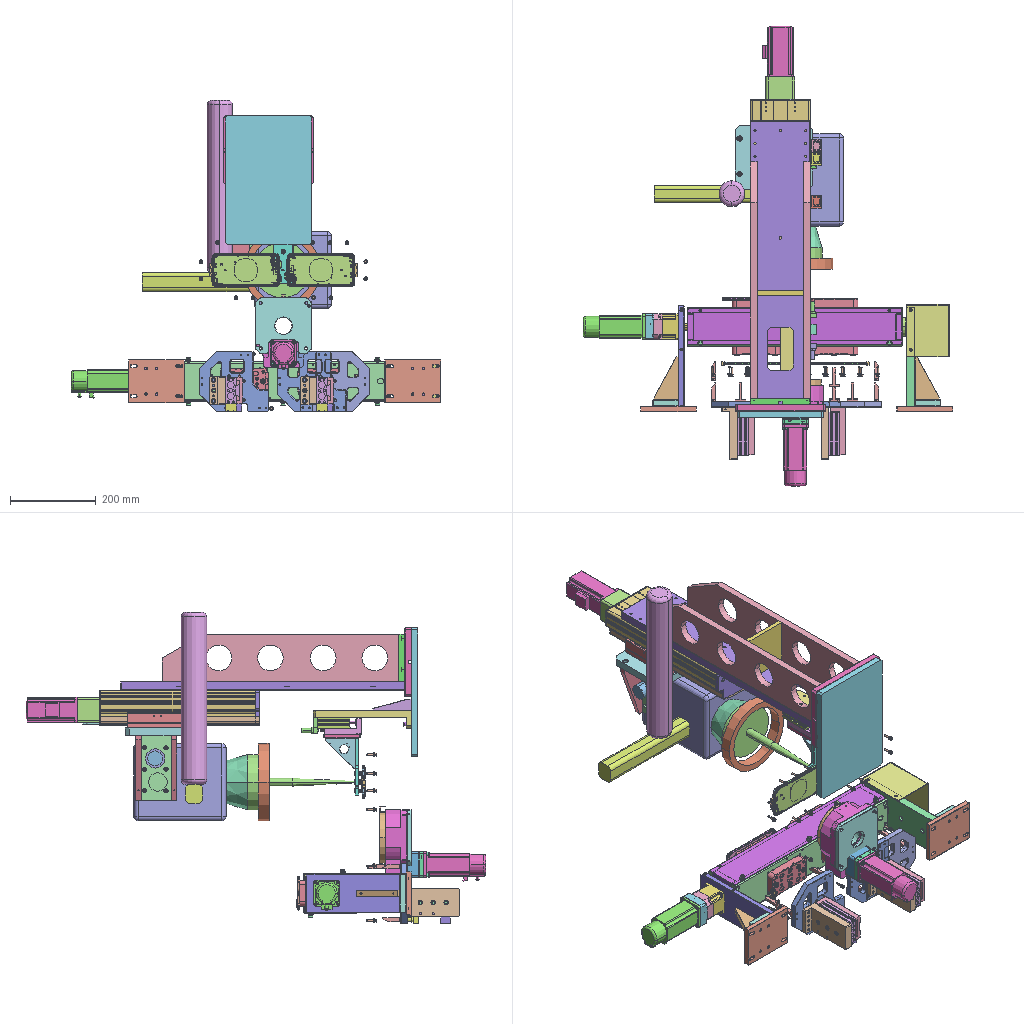Assembly | SolidWorks | 115 different items | 807 placed | box 861 x 1070 x 725 mm
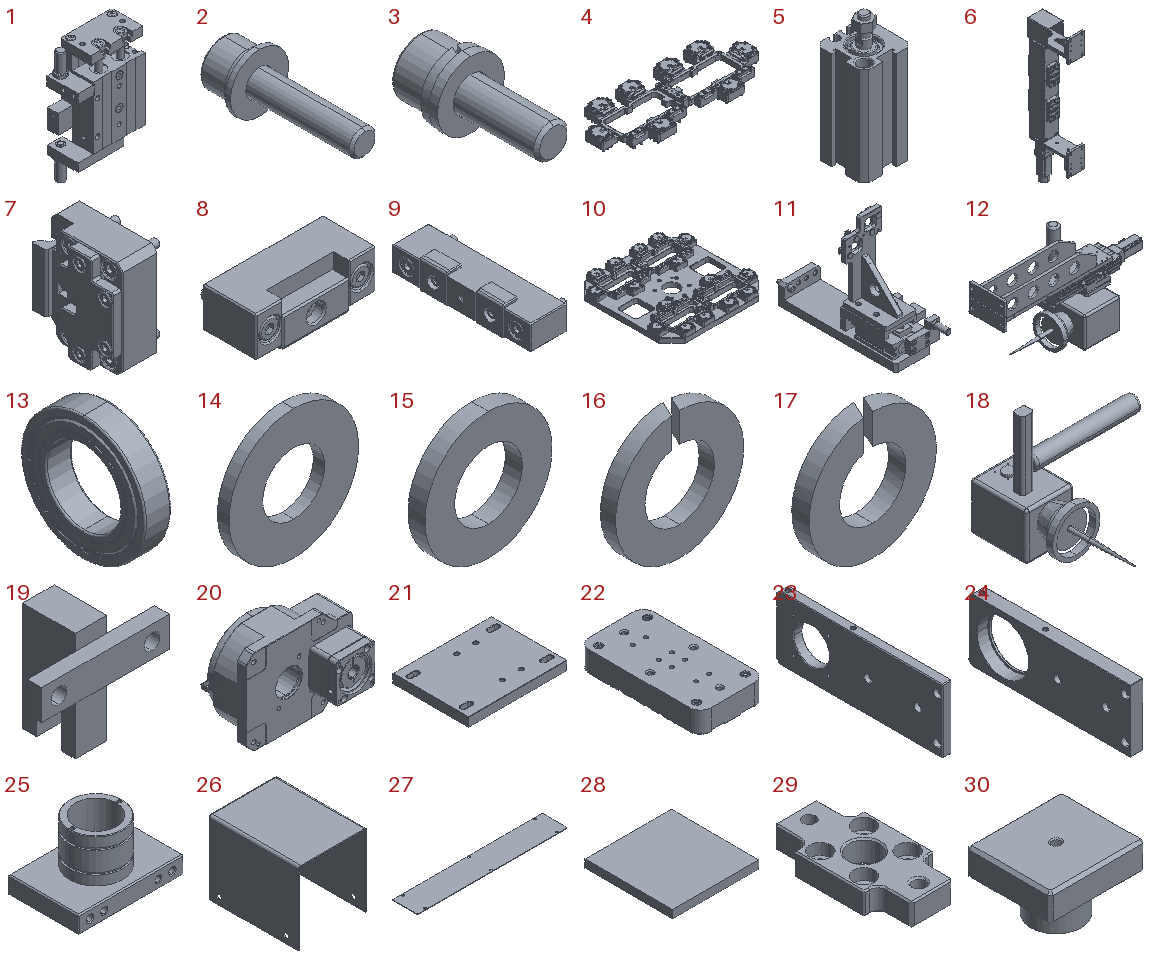Parts list (item | name | quantity | parent item | size | volume | features):
1 | (subassembly) | x1 | in 11 | 80 x 40 x 138.911 mm | 215455 mm3 | features AEMSimFeature 1, Attribute 1
2 | (subassembly) | x32 | - | 9 x 22 x 9 mm | 429.642 mm3 | features RefAxis 1
3 | (subassembly) | x6 | - | 12 x 24 x 12 mm | 1161 mm3 | features RefAxis 1
4 | (subassembly) | x2 | in 10 | - | 446882 mm3 | features Attribute 1
5 | (subassembly) | x4 | in 6 | 25 x 25.4 x 70 mm | 23906 mm3 | features Attribute 1
6 | (subassembly) | x1 | - | - | 4546068 mm3 | features ReferencePattern 103, InContextFeatHolder 53, LocalLPattern 10, CompositeCurve 8, MirrorCompFeat 3, 3DProfileFeature 1, Attribute 1, LocalCirPattern 1
7 | (subassembly) | x16 | in 4 | 29.4 x 43.863 x 50 mm | 36205 mm3 | features ReferencePattern 2, Attribute 1, CompositeCurve 1, MirrorCompFeat 1
8 | (subassembly) | x8 | in 4 | 45 x 24.4 x 17 mm | 12399 mm3 | -
9 | (subassembly) | x2 | in 4 | 26.4 x 76 x 16.4 mm | 20587 mm3 | -
10 | (subassembly) | x1 | - | - | 3131018 mm3 | features InContextFeatHolder 7, Attribute 1, LocalCirPattern 1, ReferencePattern 1
11 | (subassembly) | x1 | - | 84 x 265.5 x 198 mm | 582141 mm3 | features InContextFeatHolder 2, Attribute 1
12 | (subassembly) | x1 | - | 896.5 x 440 x 485 mm | 17056339 mm3 | features InContextFeatHolder 20, ReferencePattern 8, DerivedHolePattern 2, Attribute 1, MirrorCompFeat 1
13 | - | x1 | in 6 | 16 x 75 x 75 mm | 36953 mm3 | features BaseBody 1
14 | - | x32 | in 2 | 9 x 0.8 x 9 mm | 39.276 mm3 | features Extrusion 1, RefAxis 1
15 | - | x6 | in 3 | 12 x 1.6 x 12 mm | 129.484 mm3 | features Extrusion 1, RefAxis 1
16 | - | x32 | in 2 | 7.55 x 0.9 x 7.55 mm | 27.638 mm3 | features Extrusion 1, ICE 1, RefAxis 1
17 | - | x6 | in 3 | 11.7 x 1.6 x 11.7 mm | 121.294 mm3 | features Extrusion 1, ICE 1, RefAxis 1
18 | - | x1 | in 12 | 485 x 540 x 440 mm | 9649241 mm3 | features ICE 7, Fillet 3, Blend 1, Chamfer 1, Extrusion 1, HoleWzd 1
19 | - | x1 | in 6 | 26 x 13.7 x 22.2 mm | 1668 mm3 | features ICE 3, Extrusion 1
20 | - | x1 | - | - | - | features RefSurface 11
21 | - | x2 | in 6 | 130 x 100 x 12 mm | 148225 mm3 | features HoleWzd 2, Chamfer 1, Extrusion 1
22 | - | x4 | in 6 | 60 x 112 x 20 mm | 122613 mm3 | features Cut 6, HoleWzd 6, Chamfer 4, Extrusion 1, Fillet 1, MoveCopyBody 1
23 | - | x1 | in 6 | 13 x 234 x 90 mm | 241107 mm3 | features HoleWzd 5, Chamfer 3, ICE 2, Extrusion 1, Fillet 1, MirrorPattern 1, MoveFace 1
24 | - | x1 | in 6 | 19 x 234 x 90 mm | 311217 mm3 | features HoleWzd 6, Chamfer 3, ICE 3, Extrusion 1, Fillet 1, MoveFace 1
25 | - | x1 | in 6 | 90 x 60 x 51.6 mm | 84781 mm3 | features Chamfer 6, HoleWzd 5, ICE 5, Cut 2, Extrusion 1, MoveFace 1
26 | - | x1 | in 6 | 93.5 x 123 x 100 mm | 66221 mm3 | features Fillet 4, Cut 2, Extrusion 1, ICE 1
27 | - | x2 | in 6 | 500 x 84 x 1.5 mm | 62642 mm3 | features Cut 1, Extrusion 1, Fillet 1
28 | - | x1 | - | 108 x 110 x 10 mm | 118800 mm3 | features Extrusion 1
29 | - | x4 | in 6 | 25 x 49 x 8 mm | 5678 mm3 | features Chamfer 3, HoleWzd 3, Cut 1, Extrusion 1, Fillet 1, ICE 1
30 | - | x5 | in 6 | 17 x 15 x 11 mm | 1494 mm3 | features Chamfer 2, Extrusion 1, HoleWzd 1, ICE 1
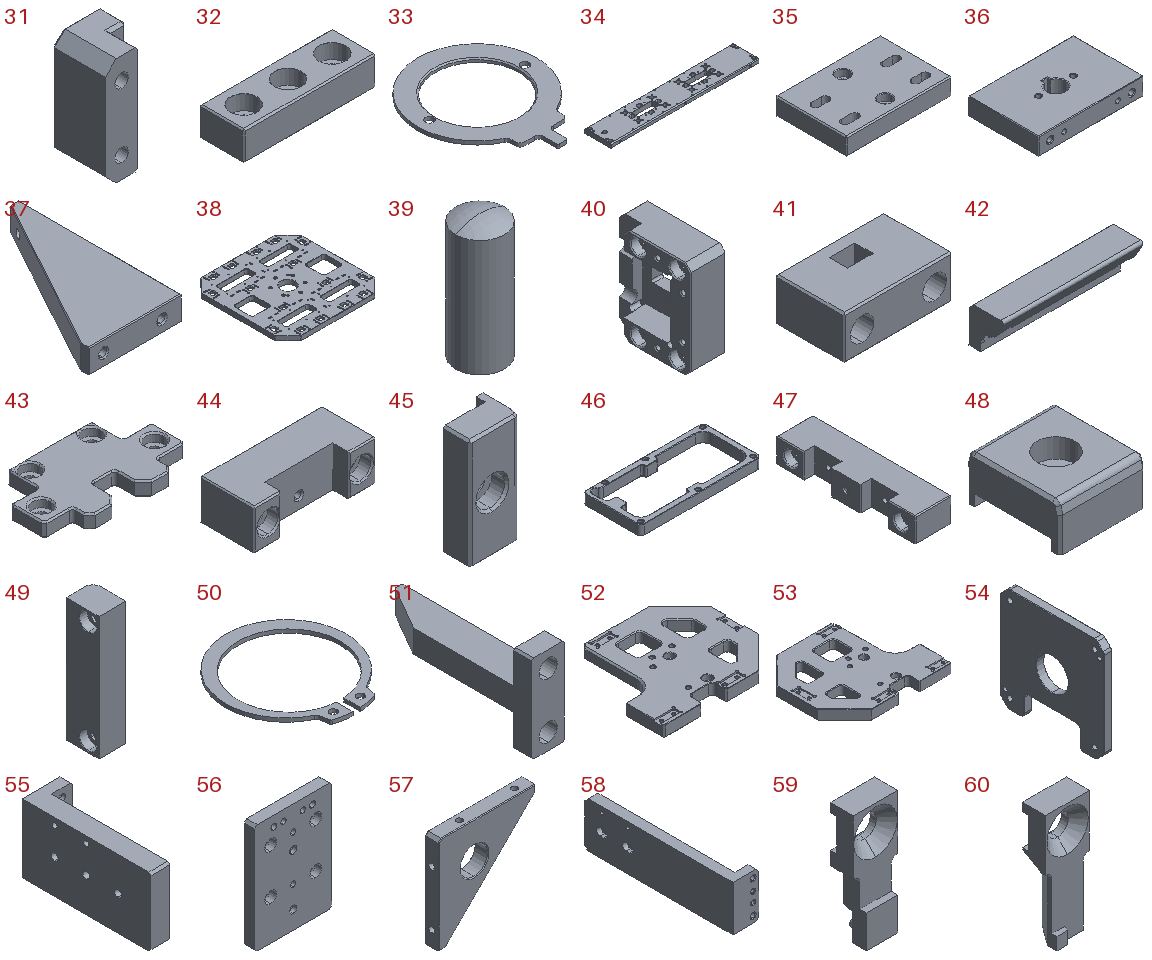31 | - | x10 | in 6 | 9 x 10 x 20 mm | 1341 mm3 | features Chamfer 2, Extrusion 1, HoleWzd 1
32 | - | x1 | in 6 | 45 x 15 x 10 mm | 5405 mm3 | features Chamfer 1, Extrusion 1, HoleWzd 1
33 | - | x2 | in 6 | 50 x 61 x 1.5 mm | 1619 mm3 | features ICE 3, Fillet 2, Chamfer 1, Extrusion 1
34 | - | x3 | in 6 | 500 x 90 x 15 mm | 566353 mm3 | features HoleWzd 8, Chamfer 5, Cut 4, LPattern 3, Extrusion 1, Fillet 1, MirrorPattern 1
35 | - | x2 | in 6 | 90 x 60 x 15 mm | 70630 mm3 | features HoleWzd 3, Chamfer 1, Extrusion 1
36 | - | x1 | in 6 | 90 x 60 x 15 mm | 75882 mm3 | features HoleWzd 3, Chamfer 2, Cut 2, Extrusion 1, ICE 1
37 | - | x2 | in 6 | 57 x 99.917 x 15 mm | 47753 mm3 | features HoleWzd 2, Chamfer 1, Extrusion 1, ICE 1
38 | - | x1 | in 10 | 420 x 420 x 20 mm | 2237254 mm3 | features HoleWzd 5, Chamfer 2, Cut 1, Extrusion 1
39 | - | x32 | in 7 | 3 x 3 x 8 mm | 53.776 mm3 | features Attribute 1, Revolution 1
40 | - | x16 | in 7 | 18 x 43 x 50 mm | 22818 mm3 | features Chamfer 5, Cut 3, HoleWzd 3, 3DProfileFeature 1, Extrusion 1
41 | - | x16 | in 7 | 30 x 19 x 12 mm | 5175 mm3 | features Chamfer 3, Cut 2, HoleWzd 2, Extrusion 1
42 | - | x16 | in 7 | 30 x 7.363 x 8 mm | 1026 mm3 | features Cut 3, Extrusion 1, HoleWzd 1
43 | - | x16 | in 7 | 50 x 29 x 5 mm | 4534 mm3 | features Chamfer 1, Extrusion 1, HoleWzd 1
44 | - | x8 | in 8 | 45 x 20 x 15 mm | 9955 mm3 | features Chamfer 4, HoleWzd 3, 3DProfileFeature 1, Extrusion 1
45 | - | x8 | in 8 | 11.5 x 8 x 25 mm | 1661 mm3 | features Chamfer 2, Extrusion 1, HoleWzd 1
46 | - | x4 | in 4 | 155.3 x 75 x 13.1 mm | 42362 mm3 | features Chamfer 2, Extrusion 1, HoleWzd 1
47 | - | x2 | in 9 | 20 x 76 x 13.6 mm | 16812 mm3 | features HoleWzd 4, Chamfer 2, Extrusion 1, ICE 1
48 | - | x4 | in 9 | 15 x 16.4 x 8 mm | 1396 mm3 | features Chamfer 1, Extrusion 1, HoleWzd 1
49 | - | x4 | - | 6.5 x 8 x 30 mm | 1393 mm3 | features HoleWzd 2, Chamfer 1, Extrusion 1, Fillet 1
50 | - | x2 | in 6 | 49 x 53.209 x 1.5 mm | 871.359 mm3 | features BaseBody 1
51 | - | x13 | - | 9 x 45 x 24.3 mm | 2894 mm3 | features ICE 3, Chamfer 2, Extrusion 1, Fillet 1
52 | - | x2 | - | 160 x 140 x 14 mm | 203256 mm3 | features Chamfer 3, Cut 2, HoleWzd 2, BaseBody 1, DelFace 1, LibraryFeature 1
53 | - | x1 | - | 160 x 140 x 14 mm | 203206 mm3 | features MoveFace 6, ICE 2, Chamfer 1, DelFace 1, HoleWzd 1, MirrorStock 1
54 | - | x1 | - | 10 x 130 x 130 mm | 133322 mm3 | features Cut 3, Chamfer 2, Fillet 2, Extrusion 1, ICE 1
55 | - | x2 | - | 38 x 122.5 x 65 mm | 149829 mm3 | features HoleWzd 4, Cut 2, ICE 2, MoveFace 2, Chamfer 1, Extrusion 1, LibraryFeature 1
56 | - | x1 | in 11 | 60 x 8 x 85 mm | 37427 mm3 | features HoleWzd 4, Chamfer 1, Extrusion 1
57 | - | x1 | in 11 | 70 x 10 x 70 mm | 23927 mm3 | features Chamfer 2, HoleWzd 2, Cut 1, Extrusion 1
58 | - | x1 | in 11 | 40 x 228 x 70 mm | 254196 mm3 | features HoleWzd 3, Chamfer 2, ICE 2, Cut 1, Extrusion 1
59 | - | x2 | in 11 | 6.75 x 4.5 x 17.8 mm | 246.564 mm3 | features Cut 6, Chamfer 2, ICE 2, Extrusion 1, Fillet 1, HoleWzd 1
60 | - | x2 | in 11 | 7 x 4.5 x 18.85 mm | 263.26 mm3 | features Cut 5, Chamfer 3, DelFace 1, Extrusion 1, Fillet 1, HoleWzd 1, MoveFace 1
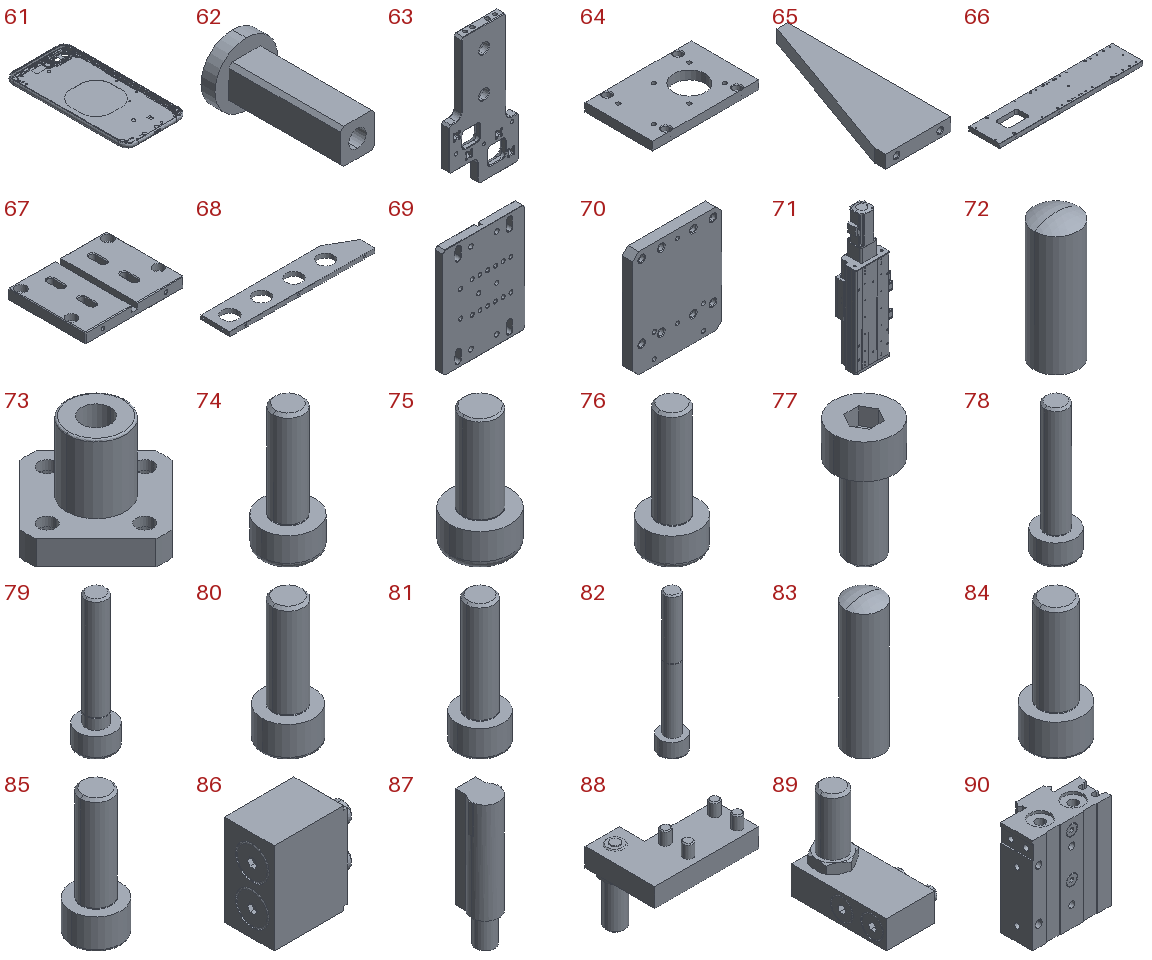61 | - | x2 | - | - | 15410 mm3 | features BaseBody 488, RefSurface 10, DeleteBody 7
62 | - | x4 | in 11 | 9 x 18 x 9 mm | 476.281 mm3 | features Chamfer 1, Extrusion 1, HoleWzd 1, ICE 1
63 | - | x1 | in 11 | 70 x 8 x 135 mm | 46021 mm3 | features MoveFace 9, Chamfer 5, Cut 4, HoleWzd 4, Fillet 2, DelFace 1, Extrusion 1, ICE 1
64 | - | x1 | in 12 | 150 x 95 x 12 mm | 144976 mm3 | features HoleWzd 2, Cut 1, Extrusion 1
65 | - | x2 | in 12 | 60 x 150 x 12 mm | 64773 mm3 | features HoleWzd 2, Extrusion 1
66 | - | x1 | in 12 | 661 x 140 x 20 mm | 1704232 mm3 | features HoleWzd 4, Cut 3, ICE 2, Chamfer 1, Extrusion 1, Fillet 1, LibraryFeature 1
67 | - | x1 | in 12 | 140 x 110 x 15 mm | 204135 mm3 | features HoleWzd 3, Chamfer 2, Cut 1, Extrusion 1, ICE 1, LibraryFeature 1
68 | - | x2 | in 12 | 550 x 110 x 16 mm | 740256 mm3 | features HoleWzd 4, ICE 4, LibraryFeature 2, Chamfer 1, Cut 1, Extrusion 1, Fillet 1
69 | - | x1 | in 12 | 160 x 15 x 210 mm | 461723 mm3 | features HoleWzd 4, Chamfer 2, Cut 2, ICE 2, LPattern 2, Extrusion 1, LibraryFeature 1
70 | - | x1 | in 12 | 150 x 18 x 180 mm | 468816 mm3 | features HoleWzd 2, Chamfer 1, Cut 1, Extrusion 1
71 | - | x1 | in 12 | 165.473 x 88 x 543.5 mm | 2791596 mm3 | features BaseBody 23
72 | - | x1 | in 11 | 4 x 4 x 12 mm | 144.223 mm3 | features Attribute 1, Revolution 1
73 | - | x16 | in 6 | 28 x 28 x 19 mm | 2991 mm3 | features BaseBody 1
74 | - | x4 | in 9 | 4.5 x 4.5 x 10.5 mm | 74.603 mm3 | features BaseBody 1
75 | - | x32 | in 7 | 3.5 x 3.5 x 7 mm | 32.905 mm3 | features Attribute 1, Cut 1, Revolution 1
76 | - | x64 | in 7 | 5.5 x 5.5 x 13 mm | 133.94 mm3 | features Attribute 1, Cut 1, Revolution 1
77 | - | x16 | in 6 | 7 x 7 x 14 mm | 241.368 mm3 | features ICE 3, Chamfer 1, Extrusion 1
78 | - | x80 | in 7, 8 | 7 x 7 x 24 mm | 391.462 mm3 | features BaseBody 1
79 | - | x4 | in 9 | 7 x 7 x 26 mm | 416.594 mm3 | features BaseBody 1
80 | - | x2 | - | 10 x 10 x 24 mm | 921.395 mm3 | features Attribute 1, Cut 1, Revolution 1
81 | - | x1 | in 11 | 10 x 10 x 28 mm | 1034 mm3 | features Attribute 1, Cut 1, Revolution 1
82 | - | x3 | - | 10 x 10 x 56 mm | 1826 mm3 | features Attribute 1, Cut 1, Revolution 1
83 | - | x2 | in 11 | 4 x 4 x 15 mm | 181.922 mm3 | features Attribute 1, Revolution 1
84 | - | x4 | in 12 | 13 x 13 x 30 mm | 2066 mm3 | features Attribute 1, Cut 1, Revolution 1
85 | - | x6 | in 12 | 13 x 13 x 33 mm | 2217 mm3 | features Attribute 1, Cut 1, Revolution 1
86 | - | x1 | in 1 | 23 x 12.5 x 23 mm | 5456 mm3 | features BaseBody 1
87 | - | x2 | in 1 | 4 x 4.8 x 18 mm | 219.808 mm3 | features BaseBody 1
88 | - | x1 | in 1 | 55 x 37.275 x 44.5 mm | 18284 mm3 | features BaseBody 1
89 | - | x1 | in 1 | 23.5 x 37.5 x 38.5 mm | 10323 mm3 | features BaseBody 1
90 | - | x1 | in 1 | 62 x 33 x 75 mm | 93823 mm3 | features BaseBody 1
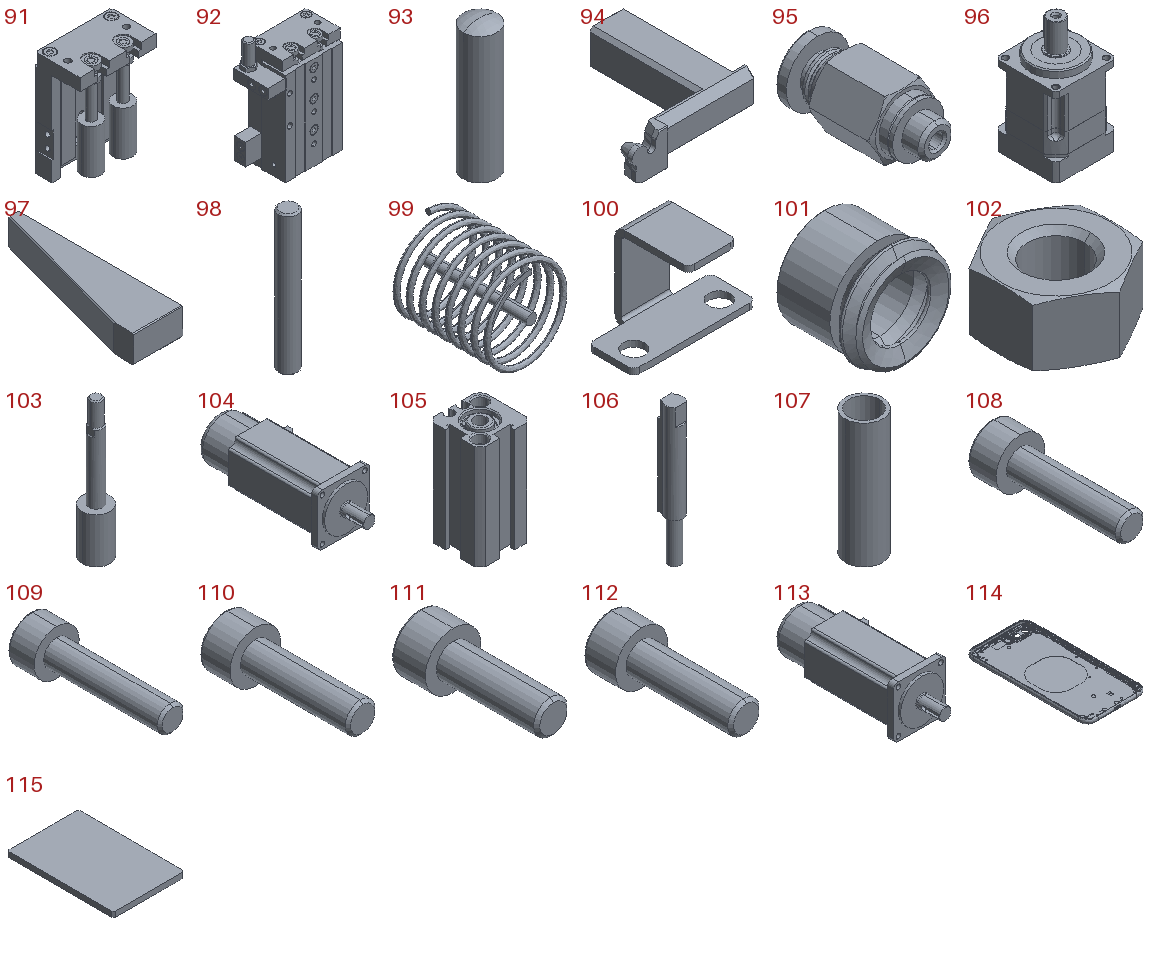91 | - | x1 | in 1 | 62 x 37 x 86 mm | 87128 mm3 | features BaseBody 1, HoleWzd 1, LibraryFeature 1, MoveFace 1
92 | - | x2 | - | 80 x 40 x 123 mm | 242427 mm3 | features BaseBody 6, HoleWzd 2, LibraryFeature 2, MoveFace 1
93 | - | x24 | in 4 | 4 x 4 x 16 mm | 194.489 mm3 | features Attribute 1, Revolution 1
94 | - | x1 | in 11 | 17.497 x 17 x 5 mm | 457.03 mm3 | features Chamfer 5, ICE 4, Cut 1, Extrusion 1, Fillet 1, HoleWzd 1
95 | - | x16 | in 6 | 10.392 x 19.5 x 9.5 mm | 848.842 mm3 | features BaseBody 1
96 | - | x1 | in 6 | 60 x 60 x 114 mm | 258118 mm3 | features ICE 22, CirPattern 8, Fillet 5, Chamfer 3, 3DProfileFeature 2, HoleWzd 2, BlendCut 1, Extrusion 1
97 | - | x2 | - | 27 x 89.833 x 15 mm | 23621 mm3 | features Chamfer 1, Extrusion 1, ICE 1
98 | - | x16 | in 6 | 6 x 6 x 45 mm | 1230 mm3 | features Chamfer 1, Extrusion 1, HoleWzd 1
99 | - | x4 | in 11 | 8.5 x 10.25 x 8.5 mm | 47.392 mm3 | features ICE 2, Helix 1, Sweep 1
100 | - | x1 | - | 20 x 12 x 14 mm | 327.403 mm3 | features EdgeFlange 2, BreakCorner 1, FlatPattern 1, SMBaseFlange 1, SheetMetal 1
101 | - | x16 | in 6 | 11.8 x 9.5 x 11.8 mm | 493.379 mm3 | features BaseBody 1
102 | - | x4 | in 5 | 8 x 9.238 x 4.5 mm | 185.536 mm3 | features BaseBody 1
103 | - | x4 | in 5 | 12 x 12 x 59.5 mm | 3239 mm3 | features BaseBody 1
104 | - | x1 | - | 69.828 x 174 x 60 mm | 379758 mm3 | features ICE 11, Fillet 6, Chamfer 2, Extrusion 1
105 | - | x4 | in 5 | 25 x 25 x 50.5 mm | 19687 mm3 | features BaseBody 1
106 | - | x8 | in 5 | 4 x 4.6 x 33.5 mm | 397.122 mm3 | features BaseBody 1
107 | - | x32 | in 7 | 6 x 6 x 20 mm | 188.338 mm3 | features Extrusion 1
108 | - | x6 | - | 7 x 20 x 7 mm | 337.596 mm3 | features ICE 2, Chamfer 1, Extrusion 1, Fillet 1, RefAxis 1
109 | - | x32 | in 2 | 7 x 22 x 7 mm | 362.728 mm3 | features ICE 2, Chamfer 1, Extrusion 1, Fillet 1, RefAxis 1
110 | - | x4 | - | 8.5 x 23 x 8.5 mm | 599.825 mm3 | features ICE 2, Chamfer 1, Extrusion 1, Fillet 1, RefAxis 1
111 | - | x6 | in 3 | 10 x 24 x 10 mm | 909.807 mm3 | features ICE 2, Chamfer 1, Extrusion 1, Fillet 1, RefAxis 1
112 | - | x8 | - | 10 x 26 x 10 mm | 966.356 mm3 | features ICE 2, Chamfer 1, Extrusion 1, Fillet 1, RefAxis 1
113 | - | x1 | in 6 | 69.828 x 174 x 60 mm | 379758 mm3 | features ICE 11, Fillet 6, Chamfer 2, Extrusion 1
114 | - | x1 | in 6 | - | 15410 mm3 | features BaseBody 488, RefSurface 10, DeleteBody 7
115 | - | x1 | - | 200 x 300 x 15 mm | 899250 mm3 | features Chamfer 1, Extrusion 1
Mates (type | each side: item.copy, entity, surface, feature), first 393 of 454 lines:
In the top assembly
Coincident | 21.1 face plane Boss-Extrude 1 | 69.1 face plane Boss-Extrude 1
Width | 41.1 face plane Cut-Extrude 2 | 41.1 face plane Cut-Extrude 2 | 51.1 face plane Boss-Extrude 1 | 51.1 face plane Boss-Extrude 1
Width | 41.2 face plane Cut-Extrude 2 | 41.2 face plane Cut-Extrude 2 | 51.2 face plane Boss-Extrude 1 | 51.2 face plane Boss-Extrude 1
Coincident | 38.1 face plane Boss-Extrude 1 | 20.1 face plane RS130-004-1-surface1
Concentric | 38.1 face cylinder Boss-Extrude 1 | 20.1 face cylinder RS130-004-1-surface1
Parallel | 38.1 face plane Boss-Extrude 1 | 20.1 face plane RS130-001-1-surface1
Symmetric | 46.1 face plane Boss-Extrude 1 | 46.1 face plane Boss-Extrude 1 | 61.1 plane
Coincident | 46.1 face plane Boss-Extrude 1 | 61.1 vertex
Parallel | 46.1 face plane Boss-Extrude 1 | 61.1 face plane PRT0509-1-1-1-solid1
Tangent | 48.1 face plane Boss-Extrude 1 | 61.1 edge
Concentric | 75.1 face cylinder Revolve1 | 49.1 face cylinder M2 六角头机械Screw的柱形沉头Hole 1
Concentric | 75.2 edge | 49.1 face cylinder M2 六角头机械Screw的柱形沉头Hole 1
Coincident | 41.3 face plane Boss-Extrude 1 | 49.1 face plane Boss-Extrude 1
Concentric | 75.3 face cylinder Revolve1 | 49.2 face cylinder M2 六角头机械Screw的柱形沉头Hole 1
Coincident | 41.4 face plane Boss-Extrude 1 | 49.2 face plane Boss-Extrude 1
Concentric | 75.4 face cylinder Revolve1 | 49.2 face cylinder M2 六角头机械Screw的柱形沉头Hole 1
Concentric | 75.5 face cylinder Revolve1 | 49.3 face cylinder M2 六角头机械Screw的柱形沉头Hole 1
Concentric | 75.6 face cylinder Revolve1 | 49.3 face cylinder M2 六角头机械Screw的柱形沉头Hole 1
Coincident | 41.2 face plane Boss-Extrude 1 | 49.3 face plane Boss-Extrude 1
Concentric | 75.7 face cylinder Revolve1 | 49.4 face cylinder M2 六角头机械Screw的柱形沉头Hole 1
Concentric | 75.8 face cylinder Revolve1 | 49.4 face cylinder M2 六角头机械Screw的柱形沉头Hole 1
Coincident | 41.5 face plane Boss-Extrude 1 | 49.4 face plane Boss-Extrude 1
Coincident | 51.3 face plane Boss-Extrude 2 | 51.4 face plane Boss-Extrude 2
Width | 51.3 face plane Boss-Extrude 1 | 51.5 face plane Boss-Extrude 1 | 52.1 face plane 输入1 | 52.1 face plane 输入1
Coincident | 51.3 face plane Boss-Extrude 2 | 52.1 face plane 输入1
Coincident | 51.4 face plane Boss-Extrude 1 | 51.6 face plane Boss-Extrude 1
Concentric | 51.4 face cylinder Cut-Extrude 2 | 52.1 face cylinder 输入1
Width | 52.1 face plane 输入1 | 52.1 face plane 输入1 | 51.5 face plane Boss-Extrude 2 | 51.6 face plane Boss-Extrude 1
Coincident | 52.1 face plane 输入1 | 92.1 face plane _MDX16x50-SG2BM1(0)_Ro-1-solid1
Concentric | 52.1 face cylinder Hole1 | 80.1 select_type:24
DistanceDim | 52.1 face plane Hole1 | 80.1 select_type:25
Coincident | 52.1 face plane 输入1 | 53.1 face plane | 2 times
DistanceDim | 55.1 face plane Boss-Extrude 1 | 52.1 face plane 输入1 | 2 times
Coincident | 52.1 face plane 输入1 | 51.7 face plane Boss-Extrude 2
Concentric | 52.1 face cylinder 输入1 | 51.6 face cylinder Cut-Extrude 2
Coincident | 55.1 face plane Boss-Extrude 1 | 92.1 face plane _MDX16x50-SG2BM1(0)_Bo-1-solid1
Width | 55.1 face plane Boss-Extrude 1 | 55.1 face plane Cut-Extrude 1 | 92.1 face plane _MDX16x50-SG2BM1(0)_Bo-1-solid1 | 92.1 face plane _MDX16x50-SG2BM1(0)_Bo-1-solid1
Concentric | 55.1 face cylinder Hole1 | 82.1 select_type:24
DistanceDim | 55.1 face plane Hole1 | 82.1 select_type:25
Coincident | 51.6 face plane Boss-Extrude 1 | 51.8 face plane Boss-Extrude 1 | 2 times
Coincident | 55.2 face plane Boss-Extrude 1 | 53.1 face plane
Coincident | 53.1 face plane | 51.1 face plane Boss-Extrude 2
Concentric | 53.1 face cylinder | 51.9 face cylinder Cut-Extrude 2
Coincident | 51.9 face plane Boss-Extrude 1 | 51.2 face plane Boss-Extrude 1 | 2 times
Coincident | 51.2 face plane Boss-Extrude 1 | 51.9 face plane Boss-Extrude 1
Coincident | 100.1 face plane Base-Flange 1 | 20.1 face plane RS130-004-1-surface1
Concentric | 100.1 face cylinder Base-Flange 1 | 20.1 face cylinder RS-130-011-1-surface1
Concentric | 20.1 face cylinder RS130-003-1-surface1 | 104.1 face cylinder Boss-Extrude 4
Parallel | 20.1 face plane RS-130-008-1-surface1 | 104.1 face plane Boss-Extrude 5
Coincident | 20.1 face plane RS-130-008-1-surface1 | 104.1 face plane Boss-Extrude 1
Concentric | 20.1 face cylinder RS130-001-1-surface1 | 54.1 face cylinder Cut-Extrude 6
Coincident | 20.1 face plane RS130-001-1-surface1 | 54.1 face plane Boss-Extrude 1 | 2 times
Coincident | 55.2 face plane Boss-Extrude 1 | 54.1 face plane Boss-Extrude 1
DistanceDim | 38.1 face plane Boss-Extrude 1 | 69.1 face plane Boss-Extrude 1
Width | 22.1 face plane Boss-Extrude 1 | 22.1 face plane Boss-Extrude 1 | 40.1 face plane Boss-Extrude 1 | 40.1 face plane Boss-Extrude 1
Parallel | 38.1 face plane Boss-Extrude 1 | 58.1 face plane Boss-Extrude 1
DistanceDim | 69.1 face plane Boss-Extrude 1 | 38.1 face plane Boss-Extrude 1
Width | 23.1 face plane Boss-Extrude1 | 24.1 face plane Boss-Extrude1 | 38.1 face plane Boss-Extrude 1 | 38.1 face plane Boss-Extrude 1
Coincident | 20.1 plane | assembly plane
Coincident | 54.1 face plane Boss-Extrude 1 | 58.1 face plane Boss-Extrude 1
Coincident | 54.1 face plane Boss-Extrude 1 | 69.1 face plane Boss-Extrude 1
Coincident | 35.1 face plane 大小六角凹头盖Screw柱Hole槽口1 | 112.1 plane
Concentric | 21.2 face cylinder M6 Tapped Hole 1 | 112.1 axis
Coincident | 35.1 face plane 大小六角凹头盖Screw柱Hole槽口1 | 112.2 plane
Concentric | 21.2 face cylinder M6 Tapped Hole 1 | 112.2 axis
Coincident | 35.1 face plane 大小六角凹头盖Screw柱Hole槽口1 | 112.3 plane
Concentric | 21.2 face cylinder M6 Tapped Hole 1 | 112.3 axis
Coincident | 35.1 face plane 大小六角凹头盖Screw柱Hole槽口1 | 112.4 plane
Concentric | 21.2 face cylinder M6 Tapped Hole 1 | 112.4 axis
Coincident | 35.2 face plane 大小六角凹头盖Screw柱Hole槽口1 | 112.5 plane
Concentric | 21.1 face cylinder M6 Tapped Hole 1 | 112.5 axis
Coincident | 35.2 face plane 大小六角凹头盖Screw柱Hole槽口1 | 112.6 plane
Concentric | 21.1 face cylinder M6 Tapped Hole 1 | 112.6 axis
Coincident | 35.2 face plane 大小六角凹头盖Screw柱Hole槽口1 | 112.7 plane
Concentric | 21.1 face cylinder M6 Tapped Hole 1 | 112.7 axis
Coincident | 35.2 face plane 大小六角凹头盖Screw柱Hole槽口1 | 112.8 plane
Concentric | 21.1 face cylinder M6 Tapped Hole 1 | 112.8 axis
Coincident | 104.1 face plane Boss-Extrude 1 | 110.1 plane
Concentric | 20.1 face cylinder RS-130-008-1-surface1 | 110.1 axis
Coincident | 104.1 face plane Boss-Extrude 1 | 110.2 plane
Concentric | 20.1 face cylinder RS-130-008-1-surface1 | 110.2 axis
Coincident | 104.1 face plane Boss-Extrude 1 | 110.3 plane
Concentric | 20.1 face cylinder RS-130-008-1-surface1 | 110.3 axis
Coincident | 104.1 face plane Boss-Extrude 1 | 110.4 plane
Concentric | 20.1 face cylinder RS-130-008-1-surface1 | 110.4 axis
Coincident | 38.1 face plane Cut-Extrude 1 | 2.1 plane
Concentric | 40.2 face cylinder 大小mm 暗销Hole 1 | 2.1 axis
Coincident | 38.1 face plane Cut-Extrude 1 | 2.2 plane
Concentric | 40.2 face cylinder 大小mm 暗销Hole 1 | 2.2 axis
Coincident | 38.1 face plane Cut-Extrude 1 | 2.3 plane
Concentric | 40.1 face cylinder 大小mm 暗销Hole 1 | 2.3 axis
Coincident | 38.1 face plane Cut-Extrude 1 | 2.4 plane
Concentric | 40.1 face cylinder 大小mm 暗销Hole 1 | 2.4 axis
Coincident | 38.1 face plane Cut-Extrude 1 | 2.5 plane
Concentric | 40.3 face cylinder 大小mm 暗销Hole 1 | 2.5 axis
Coincident | 38.1 face plane Cut-Extrude 1 | 2.6 plane
Concentric | 40.3 face cylinder 大小mm 暗销Hole 1 | 2.6 axis
Coincident | 38.1 face plane Cut-Extrude 1 | 2.7 plane
Concentric | 40.4 face cylinder 大小mm 暗销Hole 1 | 2.7 axis
Coincident | 38.1 face plane Cut-Extrude 1 | 2.8 plane
Concentric | 40.4 face cylinder 大小mm 暗销Hole 1 | 2.8 axis
Coincident | 38.1 face plane Cut-Extrude 1 | 2.9 plane
Concentric | 40.5 face cylinder 大小mm 暗销Hole 1 | 2.9 axis
Coincident | 38.1 face plane Cut-Extrude 1 | 2.10 plane
Concentric | 40.5 face cylinder 大小mm 暗销Hole 1 | 2.10 axis
Coincident | 38.1 face plane Cut-Extrude 1 | 2.11 plane
Concentric | 40.6 face cylinder 大小mm 暗销Hole 1 | 2.11 axis
Coincident | 38.1 face plane Cut-Extrude 1 | 2.12 plane
Concentric | 40.6 face cylinder 大小mm 暗销Hole 1 | 2.12 axis
Coincident | 38.1 face plane Cut-Extrude 1 | 2.13 plane
Concentric | 40.7 face cylinder 大小mm 暗销Hole 1 | 2.13 axis
Coincident | 38.1 face plane Cut-Extrude 1 | 2.14 plane
Concentric | 40.7 face cylinder 大小mm 暗销Hole 1 | 2.14 axis
Coincident | 38.1 face plane Cut-Extrude 1 | 2.15 plane
Concentric | 40.8 face cylinder 大小mm 暗销Hole 1 | 2.15 axis
Coincident | 38.1 face plane Cut-Extrude 1 | 2.16 plane
Concentric | 40.8 face cylinder 大小mm 暗销Hole 1 | 2.16 axis
Coincident | 38.1 face plane Cut-Extrude 1 | 2.17 plane
Concentric | 40.9 face cylinder 大小mm 暗销Hole 1 | 2.17 axis
Coincident | 38.1 face plane Cut-Extrude 1 | 2.18 plane
Concentric | 40.9 face cylinder 大小mm 暗销Hole 1 | 2.18 axis
Coincident | 38.1 face plane Cut-Extrude 1 | 2.19 plane
Concentric | 40.10 face cylinder 大小mm 暗销Hole 1 | 2.19 axis
Coincident | 38.1 face plane Cut-Extrude 1 | 2.20 plane
Concentric | 40.10 face cylinder 大小mm 暗销Hole 1 | 2.20 axis
Coincident | 38.1 face plane Cut-Extrude 1 | 2.21 plane
Concentric | 40.11 face cylinder 大小mm 暗销Hole 1 | 2.21 axis
Coincident | 38.1 face plane Cut-Extrude 1 | 2.22 plane
Concentric | 40.11 face cylinder 大小mm 暗销Hole 1 | 2.22 axis
Coincident | 38.1 face plane Cut-Extrude 1 | 2.23 plane
Concentric | 40.12 face cylinder 大小mm 暗销Hole 1 | 2.23 axis
Coincident | 38.1 face plane Cut-Extrude 1 | 2.24 plane
Concentric | 40.12 face cylinder 大小mm 暗销Hole 1 | 2.24 axis
Coincident | 38.1 face plane Cut-Extrude 1 | 2.25 plane
Concentric | 40.13 face cylinder 大小mm 暗销Hole 1 | 2.25 axis
Coincident | 38.1 face plane Cut-Extrude 1 | 2.26 plane
Concentric | 40.13 face cylinder 大小mm 暗销Hole 1 | 2.26 axis
Coincident | 38.1 face plane Cut-Extrude 1 | 2.27 plane
Concentric | 40.14 face cylinder 大小mm 暗销Hole 1 | 2.27 axis
Coincident | 38.1 face plane Cut-Extrude 1 | 2.28 plane
Concentric | 40.14 face cylinder 大小mm 暗销Hole 1 | 2.28 axis
Coincident | 38.1 face plane Cut-Extrude 1 | 2.29 plane
Concentric | 40.15 face cylinder 大小mm 暗销Hole 1 | 2.29 axis
Coincident | 38.1 face plane Cut-Extrude 1 | 2.30 plane
Concentric | 40.15 face cylinder 大小mm 暗销Hole 1 | 2.30 axis
Coincident | 38.1 face plane Cut-Extrude 1 | 2.31 plane
Concentric | 40.16 face cylinder 大小mm 暗销Hole 1 | 2.31 axis
Coincident | 38.1 face plane Cut-Extrude 1 | 2.32 plane
Concentric | 40.16 face cylinder 大小mm 暗销Hole 1 | 2.32 axis
Coincident | 69.1 face plane Boss-Extrude 1 | 115.1 face plane Boss-Extrude 1 | 2 times
Width | 69.1 face plane Boss-Extrude 1 | 69.1 face plane Boss-Extrude 1 | 115.1 face plane Boss-Extrude 1 | 115.1 face plane Boss-Extrude 1
Coincident | 68.1 face plane Boss-Extrude 1 | 28.1 face plane Boss-Extrude 1
Coincident | 66.1 face plane Boss-Extrude 1 | 28.1 face plane Boss-Extrude 1
DistanceDim | 28.1 face plane Boss-Extrude 1 | 67.1 face plane Boss-Extrude 1
Coincident | 58.1 face plane Boss-Extrude 1 | 97.1 face plane Boss-Extrude 1 | 2 times
Coincident | 115.1 face plane Boss-Extrude 1 | 97.1 face plane Boss-Extrude 1
Coincident | 115.1 face plane Boss-Extrude 1 | 97.2 face plane Boss-Extrude 1
Coincident | 58.1 face plane Boss-Extrude 1 | 97.2 face plane Boss-Extrude 1 | 2 times
Coincident | 51.1 face plane Boss-Extrude 2 | 108.1 plane
Concentric | 53.1 face cylinder | 108.1 axis
Coincident | 51.10 face plane Boss-Extrude 2 | 108.2 plane
Concentric | 53.1 face cylinder | 108.2 axis
Coincident | 51.10 face plane Boss-Extrude 2 | 108.3 plane
Concentric | 53.1 face cylinder | 108.3 axis
Coincident | 51.11 face plane Boss-Extrude 2 | 108.4 plane
Concentric | 53.1 face cylinder | 108.4 axis
Coincident | 51.11 face plane Boss-Extrude 2 | 108.5 plane
Concentric | 53.1 face cylinder | 108.5 axis
Coincident | 51.1 face plane Boss-Extrude 2 | 108.6 plane
Concentric | 53.1 face cylinder | 108.6 axis
Coincident | 27.1 face plane Boss-Extrude 1 | 3.1 plane
Concentric | 34.1 face cylinder M6 Tapped Hole 1 | 3.1 axis
Coincident | 27.1 face plane Boss-Extrude 1 | 3.2 plane
Concentric | 34.1 face cylinder M6 Tapped Hole 1 | 3.2 axis
Coincident | 27.1 face plane Boss-Extrude 1 | 3.3 plane
Concentric | 34.1 face cylinder M6 Tapped Hole 1 | 3.3 axis
Coincident | 27.2 face plane Boss-Extrude 1 | 3.4 plane
Concentric | 34.2 face cylinder M6 Tapped Hole 1 | 3.4 axis
Coincident | 27.2 face plane Boss-Extrude 1 | 3.5 plane
Concentric | 34.2 face cylinder M6 Tapped Hole 1 | 3.5 axis
Coincident | 27.2 face plane Boss-Extrude 1 | 3.6 plane
Concentric | 34.2 face cylinder M6 Tapped Hole 1 | 3.6 axis
In subassembly 10
Coincident | 38.2 face plane Boss-Extrude 1 | 40.17 face plane Boss-Extrude 1
Width | 40.18 face plane Boss-Extrude 1 | 40.19 face plane Boss-Extrude 1 | 38.2 face plane Boss-Extrude 1 | 38.2 face plane Boss-Extrude 1
In subassembly 4
Concentric | 93.1 face cylinder Revolve1 | 44.1 face cylinder 大小mm 暗销Hole 1
Concentric | 93.2 face cylinder Revolve1 | 44.1 face cylinder 大小mm 暗销Hole 1
Concentric | 93.3 face cylinder Revolve1 | 44.2 face cylinder 大小mm 暗销Hole 1
Concentric | 93.4 face cylinder Revolve1 | 44.2 face cylinder 大小mm 暗销Hole 1
In subassembly 7
Concentric | 40.20 face cylinder Cut-Extrude 2 | 107.1 face cylinder Boss-Extrude 1
Coincident | 40.20 face plane Cut-Extrude 2 | 107.1 face plane Boss-Extrude 1
Concentric | 40.20 face cylinder Cut-Extrude 2 | 107.2 face cylinder Boss-Extrude 1
Coincident | 40.20 face plane Cut-Extrude 2 | 107.2 face plane Boss-Extrude 1
Coincident | 40.20 face plane Cut-Extrude 1 | 41.6 face plane Boss-Extrude 1 | 2 times
Concentric | 107.1 face cylinder Boss-Extrude 1 | 41.6 face cylinder Cut-Extrude 1
Concentric | 41.6 face cylinder 大小mm 暗销Hole 0 | 42.1 face cylinder 大小mm 暗销Hole 1 | 2 times
Coincident | 41.6 face plane Boss-Extrude 1 | 42.1 face plane Boss-Extrude 1
Coincident | 40.20 face plane Boss-Extrude 1 | 43.1 face plane Boss-Extrude 1
Concentric | 40.20 face cylinder M3 Tapped Hole 1 | 43.1 face cylinder M3 六角凹头Screw的柱形沉头Hole 1 | 2 times
Concentric | 40.20 face cylinder M3 Tapped Hole 1 | 76.1 face cylinder Revolve1
Coincident | 43.1 face plane M3 六角凹头Screw的柱形沉头Hole 1 | 76.1 face plane Revolve1
Concentric | 40.20 face cylinder M3 Tapped Hole 1 | 76.2 face cylinder Revolve1
Coincident | 43.1 face plane M3 六角凹头Screw的柱形沉头Hole 1 | 76.2 face plane Revolve1
Concentric | 40.20 face cylinder M3 Tapped Hole 1 | 76.3 face cylinder Revolve1
Coincident | 43.1 face plane M3 六角凹头Screw的柱形沉头Hole 1 | 76.3 face plane Revolve1
Concentric | 40.20 face cylinder M3 Tapped Hole 1 | 76.4 face cylinder Revolve1
Coincident | 43.1 face plane M3 六角凹头Screw的柱形沉头Hole 1 | 76.4 face plane Revolve1
Concentric | 40.20 face cylinder M4 六角凹头Screw的柱形沉头Hole 1 | 78.1 face cylinder 输入1
Coincident | 40.20 face plane M4 六角凹头Screw的柱形沉头Hole 1 | 78.1 face plane 输入1
Concentric | 40.20 face cylinder M4 六角凹头Screw的柱形沉头Hole 1 | 78.2 face cylinder 输入1
Coincident | 40.20 face plane M4 六角凹头Screw的柱形沉头Hole 1 | 78.2 face plane 输入1
Concentric | 40.20 face cylinder M4 六角凹头Screw的柱形沉头Hole 1 | 78.3 face cylinder 输入1
Coincident | 40.20 face plane M4 六角凹头Screw的柱形沉头Hole 1 | 78.3 face plane 输入1
Concentric | 40.20 face cylinder M4 六角凹头Screw的柱形沉头Hole 1 | 78.4 face cylinder 输入1
Coincident | 40.20 face plane M4 六角凹头Screw的柱形沉头Hole 1 | 78.4 face plane 输入1
Concentric | 42.1 face cylinder Cut-Extrude 3 | 75.9 face cylinder Revolve1
Coincident | 42.1 face plane Boss-Extrude 1 | 75.9 face plane Revolve1
Concentric | 42.1 face cylinder 大小mm 暗销Hole 1 | 39.1 face cylinder Revolve1
Coincident | 42.1 face plane Boss-Extrude 1 | 39.1 edge
In subassembly 8
Concentric | 44.3 face cylinder M3 Tapped Hole 1 | 45.1 face cylinder M3 六角凹头Screw的柱形沉头Hole 2
Parallel | 44.3 face plane Boss-Extrude 1 | 45.1 face plane Boss-Extrude 1
Coincident | 44.3 face plane Boss-Extrude 1 | 45.1 face plane Boss-Extrude 1
Concentric | 44.3 face cylinder M4 六角凹头Screw的柱形沉头Hole 1 | 78.5 face cylinder 输入1
Coincident | 44.3 face plane M4 六角凹头Screw的柱形沉头Hole 1 | 78.5 face plane 输入1
Concentric | 44.3 face cylinder M4 六角凹头Screw的柱形沉头Hole 1 | 78.6 face cylinder 输入1
Coincident | 44.3 face plane M4 六角凹头Screw的柱形沉头Hole 1 | 78.6 face plane 输入1
In subassembly 9
Coincident | 47.1 face plane Boss-Extrude 2 | 48.2 face plane Boss-Extrude 1
Coincident | 47.1 face plane Boss-Extrude 1 | 48.2 face plane Boss-Extrude 1
Concentric | 48.2 face cylinder M3 六角凹头Screw的柱形沉头Hole 1 | 47.1 face cylinder M3 Tapped Hole 1
Coincident | 47.1 face plane Boss-Extrude 2 | 48.3 face plane Boss-Extrude 1
Coincident | 47.1 face plane Boss-Extrude 1 | 48.3 face plane Boss-Extrude 1
Concentric | 47.1 face cylinder M3 Tapped Hole 1 | 48.3 face cylinder M3 六角凹头Screw的柱形沉头Hole 1
Concentric | 47.1 face cylinder M4 六角凹头Screw的柱形沉头Hole 1 | 79.1 face cylinder 输入1
Coincident | 47.1 face plane M4 六角凹头Screw的柱形沉头Hole 1 | 79.1 face plane 输入1
Concentric | 47.1 face cylinder M4 六角凹头Screw的柱形沉头Hole 1 | 79.2 face cylinder 输入1
Coincident | 47.1 face plane M4 六角凹头Screw的柱形沉头Hole 1 | 79.2 face plane 输入1
Concentric | 47.1 face cylinder M3 Tapped Hole 1 | 74.1 face cylinder 输入1
Coincident | 48.2 face plane M3 六角凹头Screw的柱形沉头Hole 1 | 74.1 face plane 输入1
Concentric | 47.1 face cylinder M3 Tapped Hole 1 | 74.2 face cylinder 输入1
Coincident | 48.3 face plane M3 六角凹头Screw的柱形沉头Hole 1 | 74.2 face plane 输入1
In subassembly 12
Coincident | 66.2 face plane Boss-Extrude 1 | 67.2 face plane Boss-Extrude 1 | 3 times
Coincident | 66.2 face plane Boss-Extrude 1 | 68.2 face plane Boss-Extrude 1 | 2 times
Coincident | 67.2 face plane Boss-Extrude 1 | 68.3 face plane Boss-Extrude 1
Coincident | 66.2 face plane Boss-Extrude 1 | 68.3 face plane Boss-Extrude 1 | 2 times
Coincident | 67.2 face plane Boss-Extrude 1 | 68.2 face plane Boss-Extrude 1
Coincident | 67.2 face plane Boss-Extrude 1 | 69.2 face plane Boss-Extrude 1
Width | 67.2 face plane Boss-Extrude 1 | 66.2 face plane Boss-Extrude 1 | 69.2 face plane Boss-Extrude 1 | 69.2 face plane Boss-Extrude 1
Width | 67.2 face plane Boss-Extrude 1 | 67.2 face plane Boss-Extrude 1 | 69.2 face plane Boss-Extrude 1 | 69.2 face plane Boss-Extrude 1
DistanceDim | 18.1 face plane Boss-Extrude 1 | 70.1 face plane Boss-Extrude 1 | 2 times
Coincident | 66.2 face plane Boss-Extrude 1 | 71.1 face plane DG135 Base(100)-1-solid1
Parallel | 66.2 face plane Boss-Extrude 1 | 71.1 face plane DG135移动座(修改)-1-solid1
Width | 71.1 face plane DG135移动座(修改)-1-solid1 | 71.1 face plane DG135移动座(修改)-1-solid1 | 66.2 face plane Boss-Extrude 1 | 66.2 face plane Boss-Extrude 1
DistanceDim | 71.1 face plane DG135后端盖-1-solid1 | 66.2 face plane Boss-Extrude 1
DistanceDim | 18.1 face plane Boss-Extrude 1 | 71.1 face plane DG135移动座(修改)-1-solid1
Coincident | 70.1 face plane Boss-Extrude 1 | 71.1 face plane DG135移动座(修改)-1-solid1
Width | 70.1 face plane Boss-Extrude 1 | 70.1 face plane Boss-Extrude 1 | 71.1 face plane DG135移动座(修改)-1-solid1 | 71.1 face plane DG135移动座(修改)-1-solid1
Coincident | 70.1 face plane Boss-Extrude 1 | 64.1 face plane Boss-Extrude 1
Coincident | 18.1 face plane Boss-Extrude 1 | 64.1 face plane Boss-Extrude 1
DistanceDim | 18.1 face plane Boss-Extrude 1 | 64.1 face plane Boss-Extrude 1
DistanceDim | 70.1 face plane Boss-Extrude 1 | 71.1 face plane DG135移动座(修改)-1-solid1
Coincident | 64.1 face plane Boss-Extrude 1 | 65.1 face plane Boss-Extrude 1 | 2 times
Coincident | 70.1 face plane Boss-Extrude 1 | 65.1 face plane Boss-Extrude 1
Coincident | 64.1 face plane Boss-Extrude 1 | 65.2 face plane Boss-Extrude 1 | 2 times
Coincident | 70.1 face plane Boss-Extrude 1 | 65.2 face plane Boss-Extrude 1
Concentric | 67.2 face cylinder Hole1 | 84.1 select_type:24
DistanceDim | 67.2 face plane Hole1 | 84.1 select_type:25
Concentric | 66.2 face cylinder Hole1 | 85.1 select_type:24
DistanceDim | 66.2 face plane Hole1 | 85.1 select_type:25
In subassembly 6
Coincident | 36.1 face plane Boss-Extrude 1 | 34.3 face plane Boss-Extrude 1 | 3 times
Coincident | 36.1 face plane Boss-Extrude 1 | 34.4 face plane Boss-Extrude 1 | 3 times
Coincident | 34.4 face plane Boss-Extrude 1 | 22.2 face plane Boss-Extrude 1
Width | 22.2 face plane Boss-Extrude 1 | 22.2 face plane Boss-Extrude 1 | 34.4 face plane Boss-Extrude 1 | 34.4 face plane Boss-Extrude 1
Coincident | 34.4 face plane Boss-Extrude 1 | 22.3 face plane Boss-Extrude 1
Width | 22.3 face plane Boss-Extrude 1 | 22.3 face plane Boss-Extrude 1 | 34.4 face plane Boss-Extrude 1 | 34.4 face plane Boss-Extrude 1
DistanceDim | 22.2 face plane Boss-Extrude 1 | 22.3 face plane Boss-Extrude 1
Concentric | 34.4 face cylinder Cut-Extrude 1 | 73.1 face cylinder 输入1
Coincident | 34.4 face plane Boss-Extrude 1 | 73.1 face plane 输入1
Parallel | 34.4 face plane Boss-Extrude 1 | 73.1 face plane 输入1
Concentric | 73.2 face cylinder 输入1 | 98.1 face cylinder Boss-Extrude 1
DistanceDim | 98.1 face plane Boss-Extrude 1 | 22.2 face plane Boss-Extrude 1
Coincident | 34.4 face plane Boss-Extrude 1 | 29.1 face plane Boss-Extrude 1
Parallel | 22.2 face plane Boss-Extrude 1 | 30.1 face plane Boss-Extrude 2
Coincident | 22.2 face plane Boss-Extrude 1 | 30.1 face plane Boss-Extrude 2
Coincident | 22.2 face plane Boss-Extrude 1 | 31.1 face plane Boss-Extrude 1
DistanceDim | 31.1 face plane Boss-Extrude 1 | 30.1 face plane Boss-Extrude 2
Width | 31.1 face plane Boss-Extrude 1 | 31.1 face plane Boss-Extrude 1 | 22.2 face plane Boss-Extrude 1 | 22.2 face plane Boss-Extrude 1
Coincident | 22.2 face plane Boss-Extrude 1 | 31.2 face plane Boss-Extrude 1
DistanceDim | 31.2 face plane Boss-Extrude 1 | 30.1 face plane Boss-Extrude 2
Coincident | 31.1 face plane Boss-Extrude 1 | 31.2 face plane Boss-Extrude 1
Parallel | 22.4 face plane Boss-Extrude 1 | 30.2 face plane Boss-Extrude 2
Coincident | 22.4 face plane Boss-Extrude 1 | 30.2 face plane Boss-Extrude 2
Coincident | 22.4 face plane Boss-Extrude 1 | 31.3 face plane Boss-Extrude 1
DistanceDim | 31.3 face plane Boss-Extrude 1 | 30.2 face plane Boss-Extrude 2
Coincident | 22.4 face plane Boss-Extrude 1 | 31.4 face plane Boss-Extrude 1
DistanceDim | 31.4 face plane Boss-Extrude 1 | 30.2 face plane Boss-Extrude 2
Width | 31.4 face plane Boss-Extrude 1 | 31.4 face plane Boss-Extrude 1 | 30.2 face plane Boss-Extrude 2 | 30.2 face plane Boss-Extrude 2
Width | 23.2 face plane Boss-Extrude1 | 23.2 face plane Boss-Extrude1 | 36.1 face plane Boss-Extrude 1 | 36.1 face plane Boss-Extrude 1
Concentric | 23.2 face cylinder Cut-Extrude2 | 113.1 face cylinder Boss-Extrude 4
Parallel | 23.2 face plane Boss-Extrude1 | 113.1 face plane Boss-Extrude 1
Concentric | 23.2 face cylinder Cut-Extrude2 | 96.1 face cylinder Boss-Extrude 2
Coincident | 23.2 face plane Cut-Extrude1 | 96.1 face plane Boss-Extrude 1
Parallel | 23.2 face plane Boss-Extrude1 | 96.1 face plane Boss-Extrude 1
Concentric | 36.1 face cylinder Cut-Extrude 1 | 96.1 face cylinder Boss-Extrude 10
Coincident | 113.1 face plane Boss-Extrude 1 | 96.1 face plane Boss-Extrude 6
Concentric | 32.1 face cylinder 大小六角凹头盖Screw柱Hole 1 | 96.1 face cylinder Boss-Extrude 10
Parallel | 34.4 face plane Boss-Extrude 1 | 32.1 face plane Boss-Extrude 1
Coincident | 36.1 face plane Boss-Extrude 1 | 32.1 face plane Boss-Extrude 1
Parallel | 34.4 face plane Boss-Extrude 1 | 24.2 face plane Boss-Extrude1
Width | 25.1 face plane Boss-Extrude 1 | 25.1 face plane Boss-Extrude 1 | 24.2 face plane Boss-Extrude1 | 24.2 face plane Boss-Extrude1
Coincident | 34.4 face plane Boss-Extrude 1 | 25.1 face plane Boss-Extrude 1 | 3 times
Parallel | 24.2 face plane Boss-Extrude1 | 33.1 face plane Boss-Extrude 2
Coincident | 33.1 face plane Boss-Extrude 1 | 25.1 face plane Boss-Extrude 2
Concentric | 24.2 face cylinder Cut-Extrude2 | 13.1 face cylinder 输入1
Coincident | 24.2 face plane Boss-Extrude 1 | 13.1 face plane 输入1
Concentric | 25.1 face cylinder Boss-Extrude 2 | 13.1 face cylinder 输入1
DistanceDim | 24.2 face plane Boss-Extrude1 | 25.1 face plane Boss-Extrude 1
Concentric | 33.1 face cylinder Boss-Extrude 1 | 25.1 face cylinder Cut-Extrude 3
Coincident | 24.2 face plane Cut-Extrude1 | 35.3 face plane Boss-Extrude 1
Coincident | 23.2 face plane Cut-Extrude1 | 35.4 face plane Boss-Extrude 1
Coincident | 23.2 face plane Boss-Extrude1 | 35.4 face plane Boss-Extrude 1 | 2 times
Coincident | 35.4 face plane Boss-Extrude 1 | 37.1 face plane Boss-Extrude 1
Coincident | 23.2 face plane Cut-Extrude1 | 37.1 face plane Boss-Extrude 1
Width | 37.1 face plane Boss-Extrude 1 | 37.1 face plane Boss-Extrude 1 | 35.4 face plane Boss-Extrude 1 | 35.4 face plane Boss-Extrude 1
Coincident | 35.3 face plane Boss-Extrude 1 | 24.2 face plane Boss-Extrude1
Coincident | 24.2 face plane Boss-Extrude1 | 35.3 face plane Boss-Extrude 1
Coincident | 35.3 face plane Boss-Extrude 1 | 37.2 face plane Boss-Extrude 1
Coincident | 24.2 face plane Cut-Extrude1 | 37.2 face plane Boss-Extrude 1
Width | 37.2 face plane Boss-Extrude 1 | 37.2 face plane Boss-Extrude 1 | 35.3 face plane Boss-Extrude 1 | 35.3 face plane Boss-Extrude 1
Coincident | 22.3 face plane Boss-Extrude 1 | 114.1 plane
Coincident | 22.2 plane | 114.1 plane | 2 times
Coincident | 24.2 face plane Cut-Extrude1 | 19.1 face plane Boss-Extrude 1
Width | 19.1 face plane Boss-Extrude 1 | 19.1 face plane Boss-Extrude 1 | 24.2 face plane Boss-Extrude1 | 24.2 face plane Boss-Extrude1
Coincident | 24.2 face plane Boss-Extrude1 | 26.1 face plane Boss-Extrude 1
Width | 26.1 face plane Boss-Extrude 1 | 26.1 face plane Boss-Extrude 1 | 24.2 face plane Boss-Extrude1 | 24.2 face plane Boss-Extrude1
Coincident | 34.3 face plane Boss-Extrude 1 | 27.3 face plane Boss-Extrude 1
DistanceDim | 25.1 face plane Boss-Extrude 1 | 27.3 face plane Boss-Extrude 1
Coincident | 34.3 face plane Boss-Extrude 1 | 27.4 face plane Boss-Extrude 1
Concentric | 6.1 face | 77.1 face cylinder Boss-Extrude 1
Coincident | 6.1 face | 77.1 face plane Boss-Extrude 2
Coincident | 6.1 face | 77.2 face plane Boss-Extrude 2
Concentric | 6.1 face | 77.2 face cylinder Boss-Extrude 1
Coincident | 6.1 face | 77.3 face plane Boss-Extrude 2
Concentric | 6.1 face | 77.3 face cylinder Boss-Extrude 1
Coincident | 6.1 face | 77.4 face plane Boss-Extrude 2
Concentric | 6.1 face | 77.4 face cylinder Boss-Extrude 1
Coincident | 35.4 face plane Boss-Extrude 1 | 21.3 face plane Boss-Extrude 1
Width | 21.3 face plane Boss-Extrude 1 | 21.3 face plane Boss-Extrude 1 | 35.4 face plane Boss-Extrude 1 | 35.4 face plane Boss-Extrude 1
Width | 21.3 face plane Boss-Extrude 1 | 21.3 face plane Boss-Extrude 1 | 23.2 face plane Boss-Extrude1 | 35.4 face plane Boss-Extrude 1
Coincident | 35.3 face plane Boss-Extrude 1 | 21.4 face plane Boss-Extrude 1
DistanceDim | 21.4 face plane Boss-Extrude 1 | 35.3 face plane Boss-Extrude 1
Width | 35.3 face plane Boss-Extrude 1 | 35.3 face plane Boss-Extrude 1 | 21.4 face plane Boss-Extrude 1 | 21.4 face plane Boss-Extrude 1
Coincident | 21.3 face plane Boss-Extrude 1 | 21.4 face plane Boss-Extrude 1
Coincident | 96.1 face plane Boss-Extrude 10 | 32.1 face plane Boss-Extrude 1
Concentric | 29.2 edge | 103.1 face cylinder 输入1
Coincident | 29.2 face plane Boss-Extrude 1 | 105.1 face plane 输入1
Parallel | 29.2 face plane Boss-Extrude 2 | 105.1 face plane 输入1
Concentric | 29.1 face cylinder Cut-Extrude 1 | 103.2 face cylinder 输入1
Coincident | 29.1 face plane Boss-Extrude 1 | 105.2 face plane 输入1
Parallel | 29.1 face plane Boss-Extrude 2 | 105.2 face plane 输入1
Width | 34.4 face plane Boss-Extrude 1 | 34.3 face plane Boss-Extrude 1 | 27.3 face plane Boss-Extrude 1 | 27.3 face plane Boss-Extrude 1
Coincident | 27.3 face plane Boss-Extrude 1 | 27.4 face plane Boss-Extrude 1
Concentric | 24.2 face cylinder M3 Tapped Hole 1 | 19.1 face cylinder Cut-Extrude 2
DistanceDim | 26.1 face plane Boss-Extrude 1 | 21.4 face plane Boss-Extrude 1
Coincident | 25.1 face plane Boss-Extrude 1 | 34.5 face plane Boss-Extrude 1
Parallel | 36.1 face plane Boss-Extrude 1 | 34.5 face plane Boss-Extrude 1
ProfileCenter | 95.1 face plane 输入1 | 22.2 edge
ProfileCenter | 22.2 edge | 95.2 face plane 输入1
ProfileCenter | 22.2 edge | 95.3 face plane 输入1
ProfileCenter | 22.2 edge | 95.4 face plane 输入1
Coincident | 22.2 face plane Cut-Extrude 4 | 101.1 face plane 输入1
Concentric | 22.2 face cylinder M4 Tapped Hole 2 | 101.1 face cylinder 输入1
ProfileCenter | 101.2 edge | 22.2 face plane Cut-Extrude 3
ProfileCenter | 101.3 edge | 22.2 face plane Cut-Extrude 4
ProfileCenter | 101.4 edge | 22.2 face plane Cut-Extrude 3
Concentric | 34.4 face cylinder M6 Tapped Hole 2 | 27.4 face cylinder Cut-Extrude 1
Concentric | 27.4 face cylinder Cut-Extrude 1 | 34.5 face cylinder M6 Tapped Hole 1
Width | 34.4 face plane Boss-Extrude 1 | 34.4 face plane Boss-Extrude 1 | 22.3 face plane Boss-Extrude 1 | 22.2 face plane Boss-Extrude 1
Concentric | 30.3 face cylinder Boss-Extrude 1 | 103.3 face cylinder 输入1
In subassembly 11
Width | 56.1 face plane Boss-Extrude 1 | 56.1 face plane Boss-Extrude 1 | 91.1 face plane 输入1 | 91.1 face plane 输入1
Coincident | 56.1 face plane Boss-Extrude 1 | 57.1 face plane Boss-Extrude 1
Coincident | 91.1 face plane 输入1 | 56.1 face plane Boss-Extrude 1
Concentric | 91.1 face cylinder 输入1 | 56.1 face cylinder 大小六角凹头盖Screw柱Hole 1
Width | 58.2 face plane Boss-Extrude 1 | 58.2 face plane Boss-Extrude 1 | 91.1 face plane 输入1 | 91.1 face plane 输入1
Coincident | 90.1 face plane 输入1 | 58.2 face plane Boss-Extrude 1
Coincident | 88.1 face plane 输入1 | 58.2 face plane Boss-Extrude 1